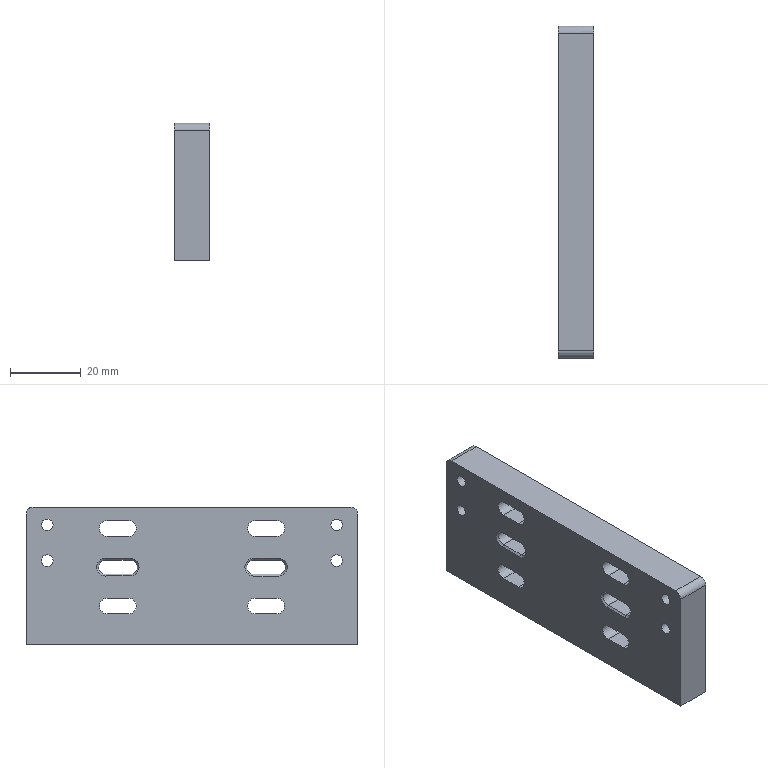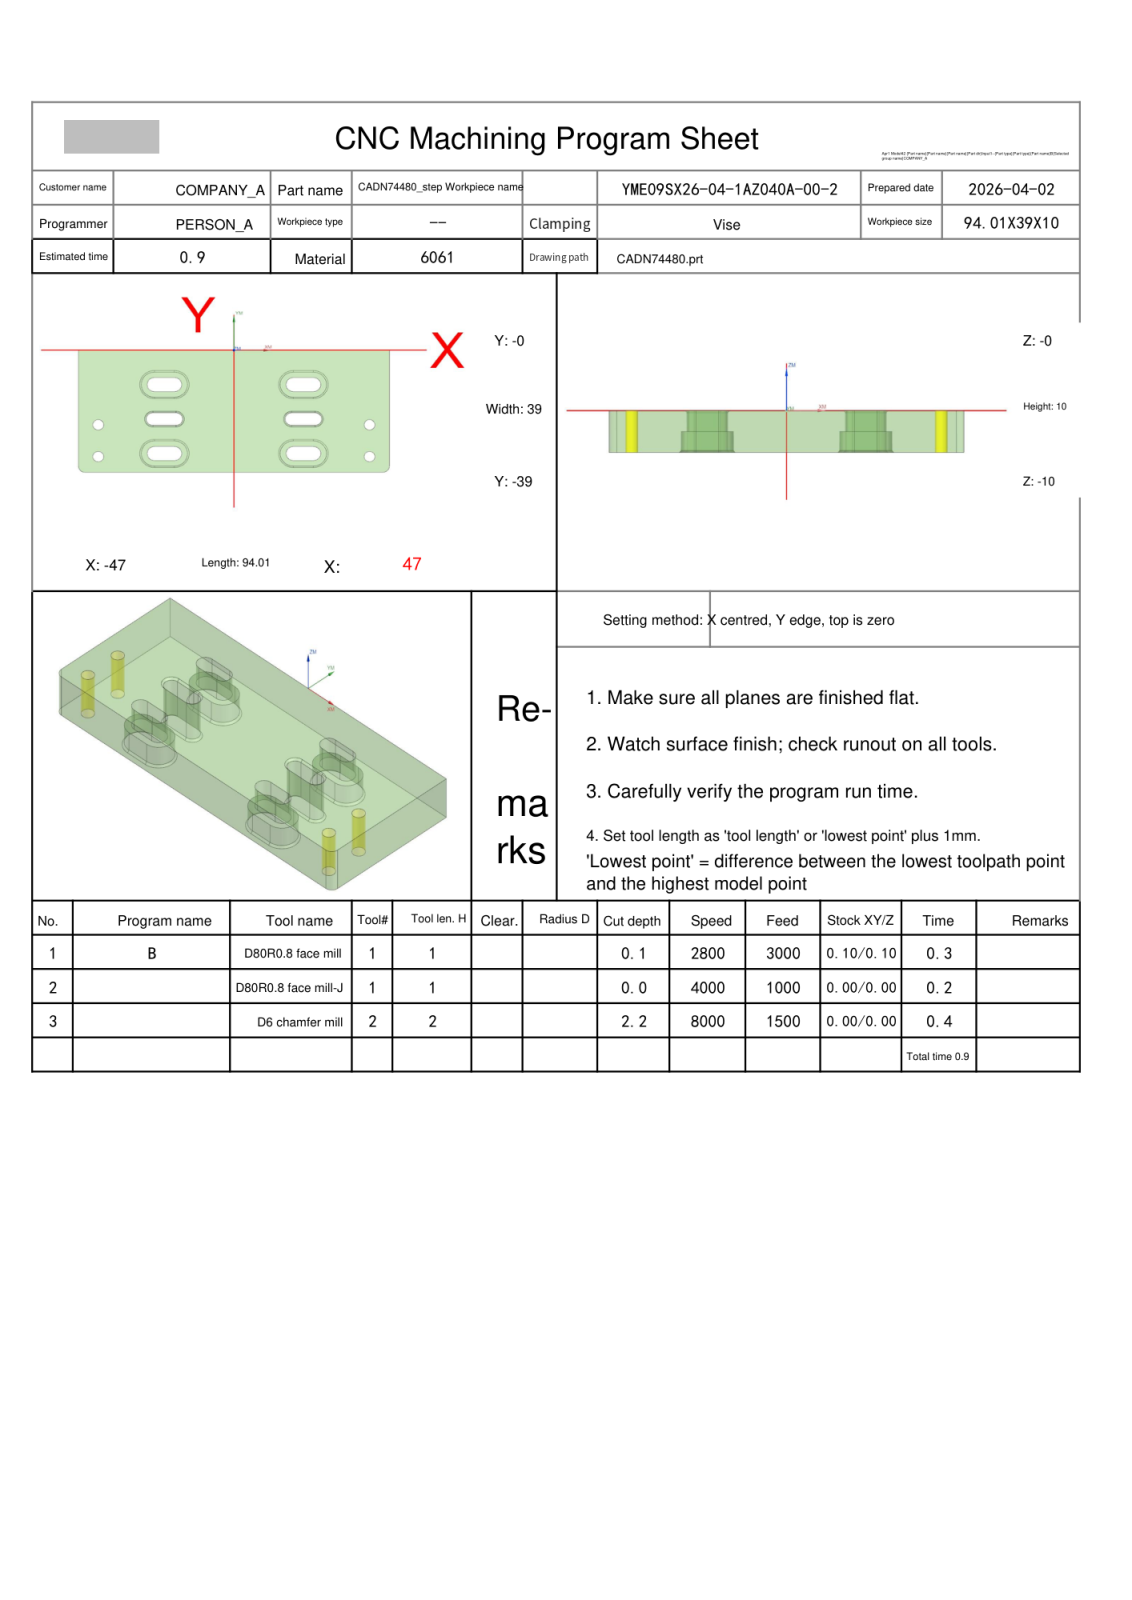NC program | NX | posted by the shop | part box 10.067 x 94 x 39 mm
Whole program:
%
O0001
(Machine time: 1.55 MIN)
(===Total Tool:2===)
(T1=D80R0.8 face mill D=80.  R=0.8  D-  H01 Z=0.    )
(T2=D6 chamfer mill   D=6.   R=0.   D-  H02 Z=-2.2  )
G80 G90 G17 G49 G40
G91 G28 Z0
M01
N1 T01 M06
(D80R0.8 face mill  D=80. R=0.8 H=01 ce=0.10 di=0.10)
G00 G90 G54 X-99.101 Y-20.797 M03 S2800
G43 H01 Z20.
M08
Z3.525
G01 Z1.525 F3000.
X-87.101 Y-20.638
X87.101 Y-18.334
X99.101 Y-18.175
Z3.525
G00 X-99.101 Y-20.797
Z3.05
G01 Z1.05
X-87.101 Y-20.638
X87.101 Y-18.334
X99.101 Y-18.175
Z3.05
G00 X-99.101 Y-20.797
Z2.575
G01 Z.575
X-87.101 Y-20.638
X87.101 Y-18.334
X99.101 Y-18.175
Z2.575
G00 X-99.101 Y-20.797
Z2.1
G01 Z.1
X-87.101 Y-20.638
X87.101 Y-18.334
X99.101 Y-18.175
Z2.1
G00 Z20.
G91 G28 Z0.0
M05
M09
G91 G28 Z0.0
M01
N2 T01 M06
(D80R0.8 face mill-J  D=80. R=0.8 H=01 ce=0.00 di=0.00)
G00 G90 G54 X-99.003 Y-20.795 M03 S4000
G43 H01 Z20.
M08
Z2.
G01 Z0.0 F1000.
X-87.003 Y-20.636
X87.003 Y-18.338
X99.003 Y-18.179
Z2.
G00 Z20.
G91 G28 Z0.0
M05
M09
G91 G28 Z0.0
M01
N3 T02 M06
(D6 chamfer mill  D=6. R=0. H=02 ce=0.00 di=0.00)
G00 G90 G54 X-40.996 Y-34. M03 S8000
G43 H02 Z20.
M08
G98 G81 X-40.996 Y-34. Z-2.2 R3. F1000.
Y-23.85
X41.004
Y-34.
G80
G00 Z20.
G00 G90 X-.389 Y1.227 M03 S6500
Z20.
Z.172
G01 Z-1.199 F1500.
G03 X-.104 Y1.027 I1.286 J1.532
G01 X-.058 Y.997
X-.004 Y1.
X46.996
G02 X47.996 Y0.0 I0.0 J-1.
G01 X47.995 Y-37.05
X47.991 Y-37.1
X47.947 Y-37.539
X47.928 Y-37.659
X47.894 Y-37.775
X47.718 Y-38.27
X47.662 Y-38.399
X47.588 Y-38.519
X47.257 Y-38.977
X47.167 Y-39.086
X47.062 Y-39.18
X46.617 Y-39.528
X46.5 Y-39.607
X46.374 Y-39.669
X45.849 Y-39.88
X45.715 Y-39.923
X45.576 Y-39.947
X45.096 Y-39.995
X45.046 Y-39.999
X-45.054
X-45.103 Y-39.995
X-45.543 Y-39.951
X-45.663 Y-39.932
X-45.779 Y-39.898
X-46.273 Y-39.722
X-46.402 Y-39.665
X-46.522 Y-39.591
X-46.981 Y-39.261
X-47.089 Y-39.17
X-47.184 Y-39.066
X-47.532 Y-38.621
X-47.611 Y-38.504
X-47.673 Y-38.377
X-47.883 Y-37.853
X-47.927 Y-37.719
X-47.95 Y-37.58
X-47.999 Y-37.1
X-48.002 Y-37.05
X-48.004 Y0.0
G02 X-47.004 Y1. I1. J0.0
G01 X-.004
X.051 Y.997
X.096 Y1.027
G03 X.382 Y1.227 I-1. J1.732
G01 Z.172
G00 Z10.
X40.585 Y-34.494
Z.402
G01 Z-1.199
G03 X40.901 Y-34.641 I1. J1.732
G01 X40.951 Y-34.662
X41.004 Y-34.65
G03 X41.654 Y-34. I0.0 J.65
X41.004 Y-33.35 I-.65 J0.0
X40.354 Y-34. I0.0 J-.65
X41.004 Y-34.65 I.65 J0.0
G01 X41.057 Y-34.662
X41.107 Y-34.641
G03 X41.423 Y-34.494 I-.684 J1.879
G01 Z.406
G00 Z2.551
X40.585 Y-24.344
Z.402
G01 Z-1.199
G03 X40.901 Y-24.491 I1. J1.732
G01 X40.951 Y-24.513
X41.004 Y-24.5
G03 X41.654 Y-23.85 I0.0 J.65
X41.004 Y-23.2 I-.65 J0.0
X40.354 Y-23.85 I0.0 J-.65
X41.004 Y-24.5 I.65 J0.0
G01 X41.057 Y-24.513
X41.107 Y-24.491
G03 X41.423 Y-24.344 I-.684 J1.879
G01 Z.406
G00 Z10.
X21.389 Y-31.977
Z.172
G01 Z-1.199
G03 X21.104 Y-31.777 I-1.286 J-1.532
G01 X21.058 Y-31.747
X21.004 Y-31.75
X18.004
G03 X16.754 Y-33. I0.0 J-1.25
X18.004 Y-34.25 I1.25 J0.0
G01 X24.004
G03 X25.254 Y-33. I0.0 J1.25
X24.004 Y-31.75 I-1.25 J0.0
G01 X21.004
X20.949 Y-31.747
X20.904 Y-31.777
G03 X20.618 Y-31.977 I1. J-1.732
G01 Z.172
G00 Z10.
X21.389 Y-9.977
Z.172
G01 Z-1.199
G03 X21.104 Y-9.777 I-1.286 J-1.532
G01 X21.058 Y-9.747
X21.004 Y-9.75
X18.004
G03 X16.754 Y-11. I0.0 J-1.25
X18.004 Y-12.25 I1.25 J0.0
G01 X24.004
G03 X25.254 Y-11. I0.0 J1.25
X24.004 Y-9.75 I-1.25 J0.0
G01 X21.004
X20.949 Y-9.747
X20.904 Y-9.777
G03 X20.618 Y-9.977 I1. J-1.732
G01 Z.172
G00 Z10.
X-20.611
Z.172
G01 Z-1.199
G03 X-20.896 Y-9.777 I-1.286 J-1.532
G01 X-20.942 Y-9.747
X-20.996 Y-9.75
X-23.996
G03 X-25.246 Y-11. I0.0 J-1.25
X-23.996 Y-12.25 I1.25 J0.0
G01 X-17.996
G03 X-16.746 Y-11. I0.0 J1.25
X-17.996 Y-9.75 I-1.25 J0.0
G01 X-20.996
X-21.051 Y-9.747
X-21.096 Y-9.777
G03 X-21.382 Y-9.977 I1. J-1.732
G01 Z.172
G00 Z10.
X-20.611 Y-31.977
Z.172
G01 Z-1.199
G03 X-20.896 Y-31.777 I-1.286 J-1.532
G01 X-20.942 Y-31.747
X-20.996 Y-31.75
X-23.996
G03 X-25.246 Y-33. I0.0 J-1.25
X-23.996 Y-34.25 I1.25 J0.0
G01 X-17.996
G03 X-16.746 Y-33. I0.0 J1.25
X-17.996 Y-31.75 I-1.25 J0.0
G01 X-20.996
X-21.051 Y-31.747
X-21.096 Y-31.777
G03 X-21.382 Y-31.977 I1. J-1.732
G01 Z.172
G00 Z10.
X-41.415 Y-34.494
Z.402
G01 Z-1.199
G03 X-41.099 Y-34.641 I1. J1.732
G01 X-41.049 Y-34.662
X-40.996 Y-34.65
G03 X-40.346 Y-34. I0.0 J.65
X-40.996 Y-33.35 I-.65 J0.0
X-41.646 Y-34. I0.0 J-.65
X-40.996 Y-34.65 I.65 J0.0
G01 X-40.943 Y-34.662
X-40.893 Y-34.641
G03 X-40.577 Y-34.494 I-.684 J1.879
G01 Z.406
G00 Z2.551
X-41.415 Y-24.344
Z.402
G01 Z-1.199
G03 X-41.099 Y-24.491 I1. J1.732
G01 X-41.049 Y-24.513
X-40.996 Y-24.5
G03 X-40.346 Y-23.85 I0.0 J.65
X-40.996 Y-23.2 I-.65 J0.0
X-41.646 Y-23.85 I0.0 J-.65
X-40.996 Y-24.5 I.65 J0.0
G01 X-40.943 Y-24.513
X-40.893 Y-24.491
G03 X-40.577 Y-24.344 I-.684 J1.879
G01 Z.406
G00 Z20.
G00 G90 X-16.678 Y-23.009 M03 S7000
Z20.
Z2.5
G01 X-16.554 Y-22.896 Z2.439 F1000.
X-16.44 Y-22.757 Z2.374
X-16.345 Y-22.604 Z2.308
X-16.273 Y-22.439 Z2.243
X-16.224 Y-22.266 Z2.177
X-16.199 Y-22.088 Z2.112
X-16.2 Y-21.908 Z2.046
X-16.225 Y-21.73 Z1.981
X-16.274 Y-21.557 Z1.915
X-16.347 Y-21.393 Z1.85
X-16.442 Y-21.24 Z1.784
X-16.557 Y-21.101 Z1.719
X-16.69 Y-20.98 Z1.653
X-16.839 Y-20.879 Z1.588
X-17. Y-20.799 Z1.523
X-17.17 Y-20.742 Z1.457
X-17.345 Y-20.709 Z1.392
X-17.526 Y-20.7 Z1.326
X-24.467 Z-1.2
X-24.496
G03 X-25.797 Y-22. I0.0 J-1.3
X-25.646 Y-22.607 I1.3 J0.0
X-24.496 Y-23.3 I1.15 J.608
G01 X-24.467
X-17.526
X-17.497
G03 X-16.196 Y-22. I0.0 J1.3
X-16.347 Y-21.393 I-1.3 J0.0
X-17.497 Y-20.7 I-1.15 J-.608
G01 X-17.526
X-24.467
X-24.65 Y-20.709
X-24.827 Y-20.742
X-24.957 Y-20.786
Z1.3
G00 Z20.
X25.322 Y-23.009
Z2.5
G01 X25.446 Y-22.896 Z2.439
X25.56 Y-22.757 Z2.374
X25.655 Y-22.604 Z2.308
X25.727 Y-22.439 Z2.243
X25.776 Y-22.266 Z2.177
X25.801 Y-22.088 Z2.112
X25.8 Y-21.908 Z2.046
X25.775 Y-21.73 Z1.981
X25.726 Y-21.557 Z1.915
X25.653 Y-21.393 Z1.85
X25.558 Y-21.24 Z1.784
X25.443 Y-21.101 Z1.719
X25.31 Y-20.98 Z1.653
X25.161 Y-20.879 Z1.588
X25. Y-20.799 Z1.523
X24.83 Y-20.742 Z1.457
X24.655 Y-20.709 Z1.392
X24.474 Y-20.7 Z1.326
X17.533 Z-1.2
X17.504
G03 X16.203 Y-22. I0.0 J-1.3
X16.354 Y-22.607 I1.3 J0.0
X17.504 Y-23.3 I1.15 J.608
G01 X17.533
X24.474
X24.503
G03 X25.804 Y-22. I0.0 J1.3
X25.653 Y-21.393 I-1.3 J0.0
X24.503 Y-20.7 I-1.15 J-.608
G01 X24.474
X17.533
X17.35 Y-20.709
X17.173 Y-20.742
X17.043 Y-20.786
Z1.3
G00 Z20.
M05
M09
G91 G28 Z0.0
G91 G28 Y0.0
M30
%